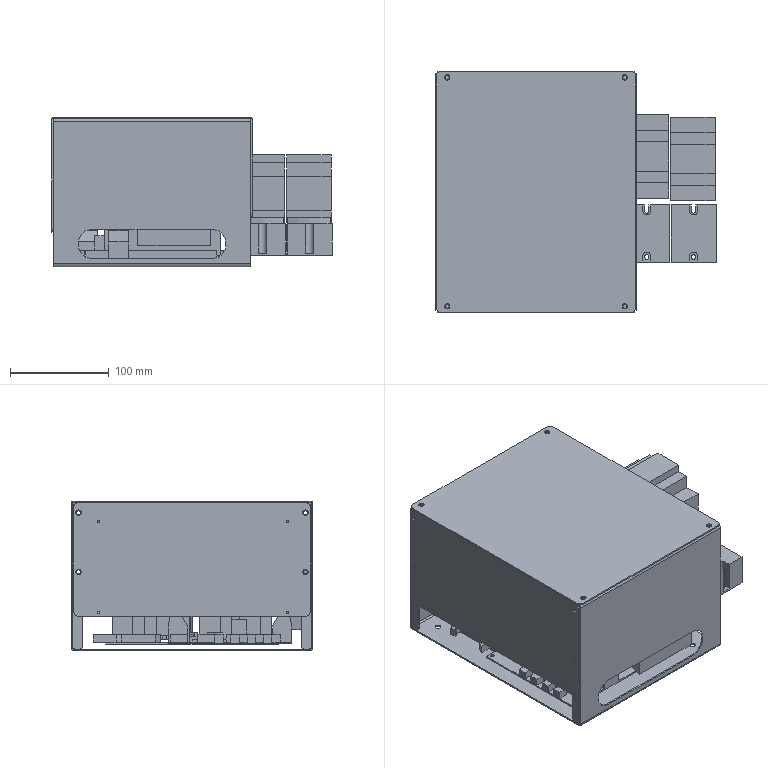Part | NX | features BREP 12 | 23 solids | 734 faces | box 284 x 245 x 151.5 mm | volume 2543766 mm3 | plane 580 | cylinder 154 | commonest cylinder face diameters 2.5 x24 3.5 x24 6 x24 10 x17 5.5 x16 4.2 x12